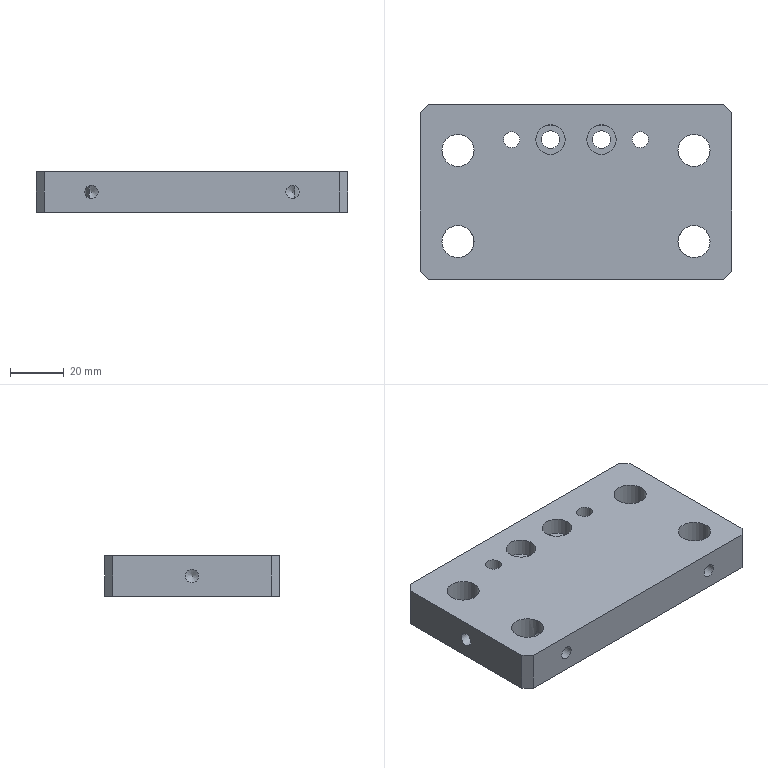Part | NX | features BREP 1 | 1 solid | 29 faces | box 116 x 65 x 15 mm | volume 102539 mm3 | cylinder 14 | plane 12 | cone 3 | commonest cylinder face diameters 5 x4 12 x4 6 x2 6.6 x2 11 x2
STEP:
#1=CARTESIAN_POINT('',(55.,-32.5,0.));
#2=VERTEX_POINT('',#1);
#3=CARTESIAN_POINT('',(58.,-29.5,0.));
#4=VERTEX_POINT('',#3);
#5=CARTESIAN_POINT('',(55.,-32.5,0.));
#6=DIRECTION('',(0.7071,0.7071,0.));
#7=VECTOR('',#6,1000.);
#8=LINE('',#5,#7);
#9=EDGE_CURVE('',#2,#4,#8,.T.);
#10=ORIENTED_EDGE('',*,*,#9,.F.);
#11=CARTESIAN_POINT('',(-55.,-32.5,0.));
#12=VERTEX_POINT('',#11);
#13=CARTESIAN_POINT('',(0.,-32.5,0.));
#14=DIRECTION('',(1.,0.,0.));
#15=VECTOR('',#14,1000.);
#16=LINE('',#13,#15);
#17=EDGE_CURVE('',#12,#2,#16,.T.);
#18=ORIENTED_EDGE('',*,*,#17,.F.);
#19=CARTESIAN_POINT('',(-58.,-29.5,0.));
#20=VERTEX_POINT('',#19);
#21=CARTESIAN_POINT('',(-58.,-29.5,0.));
#22=DIRECTION('',(0.7071,-0.7071,0.));
#23=VECTOR('',#22,1000.);
#24=LINE('',#21,#23);
#25=EDGE_CURVE('',#20,#12,#24,.T.);
#26=ORIENTED_EDGE('',*,*,#25,.F.);
#27=CARTESIAN_POINT('',(-58.,29.5,0.));
#28=VERTEX_POINT('',#27);
#29=CARTESIAN_POINT('',(-58.,0.,0.));
#30=DIRECTION('',(0.,-1.,0.));
#31=VECTOR('',#30,1000.);
#32=LINE('',#29,#31);
#33=EDGE_CURVE('',#28,#20,#32,.T.);
#34=ORIENTED_EDGE('',*,*,#33,.F.);
#35=CARTESIAN_POINT('',(-55.,32.5,0.));
#36=VERTEX_POINT('',#35);
#37=CARTESIAN_POINT('',(-55.,32.5,0.));
#38=DIRECTION('',(-0.7071,-0.7071,0.));
#39=VECTOR('',#38,1000.);
#40=LINE('',#37,#39);
#41=EDGE_CURVE('',#36,#28,#40,.T.);
#42=ORIENTED_EDGE('',*,*,#41,.F.);
#43=CARTESIAN_POINT('',(55.,32.5,0.));
#44=VERTEX_POINT('',#43);
#45=CARTESIAN_POINT('',(0.,32.5,0.));
#46=DIRECTION('',(-1.,0.,0.));
#47=VECTOR('',#46,1000.);
#48=LINE('',#45,#47);
#49=EDGE_CURVE('',#44,#36,#48,.T.);
#50=ORIENTED_EDGE('',*,*,#49,.F.);
#51=CARTESIAN_POINT('',(58.,29.5,0.));
#52=VERTEX_POINT('',#51);
#53=CARTESIAN_POINT('',(58.,29.5,0.));
#54=DIRECTION('',(-0.7071,0.7071,0.));
#55=VECTOR('',#54,1000.);
#56=LINE('',#53,#55);
#57=EDGE_CURVE('',#52,#44,#56,.T.);
#58=ORIENTED_EDGE('',*,*,#57,.F.);
#59=CARTESIAN_POINT('',(58.,0.,0.));
#60=DIRECTION('',(0.,1.,0.));
#61=VECTOR('',#60,1000.);
#62=LINE('',#59,#61);
#63=EDGE_CURVE('',#4,#52,#62,.T.);
#64=ORIENTED_EDGE('',*,*,#63,.F.);
#65=EDGE_LOOP('',(#10,#18,#26,#34,#42,#50,#58,#64));
#66=FACE_BOUND('',#65,.T.);
#67=CARTESIAN_POINT('',(38.,15.5,0.));
#68=VERTEX_POINT('',#67);
#69=CARTESIAN_POINT('',(44.,15.5,0.));
#70=DIRECTION('',(0.,0.,-1.));
#71=DIRECTION('',(-1.,0.,0.));
#72=AXIS2_PLACEMENT_3D('',#69,#70,#71);
#73=CIRCLE('',#72,6.);
#74=EDGE_CURVE('',#68,#68,#73,.T.);
#75=ORIENTED_EDGE('',*,*,#74,.F.);
#76=EDGE_LOOP('',(#75));
#77=FACE_BOUND('',#76,.T.);
#78=CARTESIAN_POINT('',(38.,-18.5,0.));
#79=VERTEX_POINT('',#78);
#80=CARTESIAN_POINT('',(44.,-18.5,0.));
#81=DIRECTION('',(0.,0.,-1.));
#82=DIRECTION('',(-1.,0.,0.));
#83=AXIS2_PLACEMENT_3D('',#80,#81,#82);
#84=CIRCLE('',#83,6.);
#85=EDGE_CURVE('',#79,#79,#84,.T.);
#86=ORIENTED_EDGE('',*,*,#85,.F.);
#87=EDGE_LOOP('',(#86));
#88=FACE_BOUND('',#87,.T.);
#89=CARTESIAN_POINT('',(-50.,-18.5,0.));
#90=VERTEX_POINT('',#89);
#91=CARTESIAN_POINT('',(-44.,-18.5,0.));
#92=DIRECTION('',(0.,0.,-1.));
#93=DIRECTION('',(-1.,0.,0.));
#94=AXIS2_PLACEMENT_3D('',#91,#92,#93);
#95=CIRCLE('',#94,6.);
#96=EDGE_CURVE('',#90,#90,#95,.T.);
#97=ORIENTED_EDGE('',*,*,#96,.F.);
#98=EDGE_LOOP('',(#97));
#99=FACE_BOUND('',#98,.T.);
#100=CARTESIAN_POINT('',(-50.,15.5,0.));
#101=VERTEX_POINT('',#100);
#102=CARTESIAN_POINT('',(-44.,15.5,0.));
#103=DIRECTION('',(0.,0.,-1.));
#104=DIRECTION('',(-1.,0.,0.));
#105=AXIS2_PLACEMENT_3D('',#102,#103,#104);
#106=CIRCLE('',#105,6.);
#107=EDGE_CURVE('',#101,#101,#106,.T.);
#108=ORIENTED_EDGE('',*,*,#107,.F.);
#109=EDGE_LOOP('',(#108));
#110=FACE_BOUND('',#109,.T.);
#111=CARTESIAN_POINT('',(21.,19.5,0.));
#112=VERTEX_POINT('',#111);
#113=CARTESIAN_POINT('',(24.,19.5,0.));
#114=DIRECTION('',(0.,0.,-1.));
#115=DIRECTION('',(-1.,0.,0.));
#116=AXIS2_PLACEMENT_3D('',#113,#114,#115);
#117=CIRCLE('',#116,3.);
#118=EDGE_CURVE('',#112,#112,#117,.T.);
#119=ORIENTED_EDGE('',*,*,#118,.F.);
#120=EDGE_LOOP('',(#119));
#121=FACE_BOUND('',#120,.T.);
#122=CARTESIAN_POINT('',(-27.,19.5,0.));
#123=VERTEX_POINT('',#122);
#124=CARTESIAN_POINT('',(-24.,19.5,0.));
#125=DIRECTION('',(0.,0.,-1.));
#126=DIRECTION('',(-1.,0.,0.));
#127=AXIS2_PLACEMENT_3D('',#124,#125,#126);
#128=CIRCLE('',#127,3.);
#129=EDGE_CURVE('',#123,#123,#128,.T.);
#130=ORIENTED_EDGE('',*,*,#129,.F.);
#131=EDGE_LOOP('',(#130));
#132=FACE_BOUND('',#131,.T.);
#133=CARTESIAN_POINT('',(12.8,19.5,0.));
#134=VERTEX_POINT('',#133);
#135=CARTESIAN_POINT('',(9.5,19.5,0.));
#136=DIRECTION('',(0.,0.,-1.));
#137=DIRECTION('',(1.,0.,0.));
#138=AXIS2_PLACEMENT_3D('',#135,#136,#137);
#139=CIRCLE('',#138,3.3);
#140=EDGE_CURVE('',#134,#134,#139,.T.);
#141=ORIENTED_EDGE('',*,*,#140,.F.);
#142=EDGE_LOOP('',(#141));
#143=FACE_BOUND('',#142,.T.);
#144=CARTESIAN_POINT('',(-6.2,19.5,0.));
#145=VERTEX_POINT('',#144);
#146=CARTESIAN_POINT('',(-9.5,19.5,0.));
#147=DIRECTION('',(0.,0.,-1.));
#148=DIRECTION('',(1.,0.,0.));
#149=AXIS2_PLACEMENT_3D('',#146,#147,#148);
#150=CIRCLE('',#149,3.3);
#151=EDGE_CURVE('',#145,#145,#150,.T.);
#152=ORIENTED_EDGE('',*,*,#151,.F.);
#153=EDGE_LOOP('',(#152));
#154=FACE_BOUND('',#153,.T.);
#155=CARTESIAN_POINT('',(0.,0.,0.));
#156=DIRECTION('',(0.,0.,1.));
#157=DIRECTION('',(-1.,0.,0.));
#158=AXIS2_PLACEMENT_3D('',#155,#156,#157);
#159=PLANE('',#158);
#160=ADVANCED_FACE('',(#66,#77,#88,#99,#110,#121,#132,#143,#154),#159,.F.);
#161=CARTESIAN_POINT('',(58.,-29.5,15.));
#162=VERTEX_POINT('',#161);
#163=CARTESIAN_POINT('',(58.,-29.5,15.));
#164=DIRECTION('',(0.,0.,1.));
#165=VECTOR('',#164,1000.);
#166=LINE('',#163,#165);
#167=EDGE_CURVE('',#4,#162,#166,.T.);
#168=ORIENTED_EDGE('',*,*,#167,.F.);
#169=ORIENTED_EDGE('',*,*,#63,.T.);
#170=CARTESIAN_POINT('',(58.,29.5,15.));
#171=VERTEX_POINT('',#170);
#172=CARTESIAN_POINT('',(58.,29.5,15.));
#173=DIRECTION('',(0.,0.,-1.));
#174=VECTOR('',#173,1000.);
#175=LINE('',#172,#174);
#176=EDGE_CURVE('',#171,#52,#175,.T.);
#177=ORIENTED_EDGE('',*,*,#176,.F.);
#178=CARTESIAN_POINT('',(58.,32.5,15.));
#179=DIRECTION('',(0.,1.,0.));
#180=VECTOR('',#179,1000.);
#181=LINE('',#178,#180);
#182=EDGE_CURVE('',#162,#171,#181,.T.);
#183=ORIENTED_EDGE('',*,*,#182,.F.);
#184=EDGE_LOOP('',(#168,#169,#177,#183));
#185=FACE_BOUND('',#184,.T.);
#186=CARTESIAN_POINT('',(58.,32.5,15.));
#187=DIRECTION('',(-1.,0.,0.));
#188=DIRECTION('',(0.,1.,0.));
#189=AXIS2_PLACEMENT_3D('',#186,#187,#188);
#190=PLANE('',#189);
#191=ADVANCED_FACE('',(#185),#190,.F.);
#192=CARTESIAN_POINT('',(55.,-32.5,15.));
#193=VERTEX_POINT('',#192);
#194=CARTESIAN_POINT('',(55.,-32.5,15.));
#195=DIRECTION('',(0.,0.,1.));
#196=VECTOR('',#195,1000.);
#197=LINE('',#194,#196);
#198=EDGE_CURVE('',#2,#193,#197,.T.);
#199=ORIENTED_EDGE('',*,*,#198,.F.);
#200=ORIENTED_EDGE('',*,*,#9,.T.);
#201=ORIENTED_EDGE('',*,*,#167,.T.);
#202=CARTESIAN_POINT('',(58.,-29.5,15.));
#203=DIRECTION('',(0.7071,0.7071,0.));
#204=VECTOR('',#203,1000.);
#205=LINE('',#202,#204);
#206=EDGE_CURVE('',#193,#162,#205,.T.);
#207=ORIENTED_EDGE('',*,*,#206,.F.);
#208=EDGE_LOOP('',(#199,#200,#201,#207));
#209=FACE_BOUND('',#208,.T.);
#210=CARTESIAN_POINT('',(58.,-29.5,15.));
#211=DIRECTION('',(-0.7071,0.7071,0.));
#212=DIRECTION('',(0.7071,0.7071,0.));
#213=AXIS2_PLACEMENT_3D('',#210,#211,#212);
#214=PLANE('',#213);
#215=ADVANCED_FACE('',(#209),#214,.F.);
#216=ORIENTED_EDGE('',*,*,#198,.T.);
#217=CARTESIAN_POINT('',(-55.,-32.5,15.));
#218=VERTEX_POINT('',#217);
#219=CARTESIAN_POINT('',(-58.,-32.5,15.));
#220=DIRECTION('',(1.,0.,0.));
#221=VECTOR('',#220,1000.);
#222=LINE('',#219,#221);
#223=EDGE_CURVE('',#218,#193,#222,.T.);
#224=ORIENTED_EDGE('',*,*,#223,.F.);
#225=CARTESIAN_POINT('',(-55.,-32.5,15.));
#226=DIRECTION('',(0.,0.,1.));
#227=VECTOR('',#226,1000.);
#228=LINE('',#225,#227);
#229=EDGE_CURVE('',#12,#218,#228,.T.);
#230=ORIENTED_EDGE('',*,*,#229,.F.);
#231=ORIENTED_EDGE('',*,*,#17,.T.);
#232=EDGE_LOOP('',(#216,#224,#230,#231));
#233=FACE_BOUND('',#232,.T.);
#234=CARTESIAN_POINT('',(-37.5,-32.5,5.));
#235=VERTEX_POINT('',#234);
#236=CARTESIAN_POINT('',(-37.5,-32.5,7.5));
#237=DIRECTION('',(0.,-1.,0.));
#238=DIRECTION('',(0.,0.,-1.));
#239=AXIS2_PLACEMENT_3D('',#236,#237,#238);
#240=CIRCLE('',#239,2.5);
#241=EDGE_CURVE('',#235,#235,#240,.T.);
#242=ORIENTED_EDGE('',*,*,#241,.F.);
#243=EDGE_LOOP('',(#242));
#244=FACE_BOUND('',#243,.T.);
#245=CARTESIAN_POINT('',(37.5,-32.5,5.));
#246=VERTEX_POINT('',#245);
#247=CARTESIAN_POINT('',(37.5,-32.5,7.5));
#248=DIRECTION('',(0.,-1.,0.));
#249=DIRECTION('',(0.,0.,-1.));
#250=AXIS2_PLACEMENT_3D('',#247,#248,#249);
#251=CIRCLE('',#250,2.5);
#252=EDGE_CURVE('',#246,#246,#251,.T.);
#253=ORIENTED_EDGE('',*,*,#252,.F.);
#254=EDGE_LOOP('',(#253));
#255=FACE_BOUND('',#254,.T.);
#256=CARTESIAN_POINT('',(-58.,-32.5,15.));
#257=DIRECTION('',(0.,1.,0.));
#258=DIRECTION('',(0.,0.,-1.));
#259=AXIS2_PLACEMENT_3D('',#256,#257,#258);
#260=PLANE('',#259);
#261=ADVANCED_FACE('',(#233,#244,#255),#260,.F.);
#262=CARTESIAN_POINT('',(-58.,-29.5,15.));
#263=VERTEX_POINT('',#262);
#264=CARTESIAN_POINT('',(-58.,-29.5,15.));
#265=DIRECTION('',(0.,0.,1.));
#266=VECTOR('',#265,1000.);
#267=LINE('',#264,#266);
#268=EDGE_CURVE('',#20,#263,#267,.T.);
#269=ORIENTED_EDGE('',*,*,#268,.F.);
#270=ORIENTED_EDGE('',*,*,#25,.T.);
#271=ORIENTED_EDGE('',*,*,#229,.T.);
#272=CARTESIAN_POINT('',(-55.,-32.5,15.));
#273=DIRECTION('',(0.7071,-0.7071,0.));
#274=VECTOR('',#273,1000.);
#275=LINE('',#272,#274);
#276=EDGE_CURVE('',#263,#218,#275,.T.);
#277=ORIENTED_EDGE('',*,*,#276,.F.);
#278=EDGE_LOOP('',(#269,#270,#271,#277));
#279=FACE_BOUND('',#278,.T.);
#280=CARTESIAN_POINT('',(-55.,-32.5,15.));
#281=DIRECTION('',(0.7071,0.7071,0.));
#282=DIRECTION('',(0.7071,-0.7071,0.));
#283=AXIS2_PLACEMENT_3D('',#280,#281,#282);
#284=PLANE('',#283);
#285=ADVANCED_FACE('',(#279),#284,.F.);
#286=CARTESIAN_POINT('',(-58.,29.5,15.));
#287=VERTEX_POINT('',#286);
#288=CARTESIAN_POINT('',(-58.,29.5,15.));
#289=DIRECTION('',(0.,0.,1.));
#290=VECTOR('',#289,1000.);
#291=LINE('',#288,#290);
#292=EDGE_CURVE('',#28,#287,#291,.T.);
#293=ORIENTED_EDGE('',*,*,#292,.F.);
#294=ORIENTED_EDGE('',*,*,#33,.T.);
#295=ORIENTED_EDGE('',*,*,#268,.T.);
#296=CARTESIAN_POINT('',(-58.,32.5,15.));
#297=DIRECTION('',(0.,-1.,0.));
#298=VECTOR('',#297,1000.);
#299=LINE('',#296,#298);
#300=EDGE_CURVE('',#287,#263,#299,.T.);
#301=ORIENTED_EDGE('',*,*,#300,.F.);
#302=EDGE_LOOP('',(#293,#294,#295,#301));
#303=FACE_BOUND('',#302,.T.);
#304=CARTESIAN_POINT('',(-58.,0.,10.));
#305=VERTEX_POINT('',#304);
#306=CARTESIAN_POINT('',(-58.,0.,7.5));
#307=DIRECTION('',(-1.,0.,0.));
#308=DIRECTION('',(0.,0.,1.));
#309=AXIS2_PLACEMENT_3D('',#306,#307,#308);
#310=CIRCLE('',#309,2.5);
#311=EDGE_CURVE('',#305,#305,#310,.T.);
#312=ORIENTED_EDGE('',*,*,#311,.F.);
#313=EDGE_LOOP('',(#312));
#314=FACE_BOUND('',#313,.T.);
#315=CARTESIAN_POINT('',(-58.,32.5,15.));
#316=DIRECTION('',(1.,0.,0.));
#317=DIRECTION('',(0.,-1.,0.));
#318=AXIS2_PLACEMENT_3D('',#315,#316,#317);
#319=PLANE('',#318);
#320=ADVANCED_FACE('',(#303,#314),#319,.F.);
#321=CARTESIAN_POINT('',(-55.,32.5,15.));
#322=VERTEX_POINT('',#321);
#323=CARTESIAN_POINT('',(-55.,32.5,15.));
#324=DIRECTION('',(0.,0.,1.));
#325=VECTOR('',#324,1000.);
#326=LINE('',#323,#325);
#327=EDGE_CURVE('',#36,#322,#326,.T.);
#328=ORIENTED_EDGE('',*,*,#327,.F.);
#329=ORIENTED_EDGE('',*,*,#41,.T.);
#330=ORIENTED_EDGE('',*,*,#292,.T.);
#331=CARTESIAN_POINT('',(-58.,29.5,15.));
#332=DIRECTION('',(-0.7071,-0.7071,0.));
#333=VECTOR('',#332,1000.);
#334=LINE('',#331,#333);
#335=EDGE_CURVE('',#322,#287,#334,.T.);
#336=ORIENTED_EDGE('',*,*,#335,.F.);
#337=EDGE_LOOP('',(#328,#329,#330,#336));
#338=FACE_BOUND('',#337,.T.);
#339=CARTESIAN_POINT('',(-58.,29.5,15.));
#340=DIRECTION('',(0.7071,-0.7071,0.));
#341=DIRECTION('',(-0.7071,-0.7071,0.));
#342=AXIS2_PLACEMENT_3D('',#339,#340,#341);
#343=PLANE('',#342);
#344=ADVANCED_FACE('',(#338),#343,.F.);
#345=CARTESIAN_POINT('',(55.,32.5,15.));
#346=VERTEX_POINT('',#345);
#347=CARTESIAN_POINT('',(55.,32.5,15.));
#348=DIRECTION('',(0.,0.,1.));
#349=VECTOR('',#348,1000.);
#350=LINE('',#347,#349);
#351=EDGE_CURVE('',#44,#346,#350,.T.);
#352=ORIENTED_EDGE('',*,*,#351,.F.);
#353=ORIENTED_EDGE('',*,*,#49,.T.);
#354=ORIENTED_EDGE('',*,*,#327,.T.);
#355=CARTESIAN_POINT('',(-58.,32.5,15.));
#356=DIRECTION('',(-1.,0.,0.));
#357=VECTOR('',#356,1000.);
#358=LINE('',#355,#357);
#359=EDGE_CURVE('',#346,#322,#358,.T.);
#360=ORIENTED_EDGE('',*,*,#359,.F.);
#361=EDGE_LOOP('',(#352,#353,#354,#360));
#362=FACE_BOUND('',#361,.T.);
#363=CARTESIAN_POINT('',(-58.,32.5,15.));
#364=DIRECTION('',(0.,-1.,0.));
#365=DIRECTION('',(0.,0.,1.));
#366=AXIS2_PLACEMENT_3D('',#363,#364,#365);
#367=PLANE('',#366);
#368=ADVANCED_FACE('',(#362),#367,.F.);
#369=ORIENTED_EDGE('',*,*,#176,.T.);
#370=ORIENTED_EDGE('',*,*,#57,.T.);
#371=ORIENTED_EDGE('',*,*,#351,.T.);
#372=CARTESIAN_POINT('',(55.,32.5,15.));
#373=DIRECTION('',(-0.7071,0.7071,0.));
#374=VECTOR('',#373,1000.);
#375=LINE('',#372,#374);
#376=EDGE_CURVE('',#171,#346,#375,.T.);
#377=ORIENTED_EDGE('',*,*,#376,.F.);
#378=EDGE_LOOP('',(#369,#370,#371,#377));
#379=FACE_BOUND('',#378,.T.);
#380=CARTESIAN_POINT('',(55.,32.5,15.));
#381=DIRECTION('',(-0.7071,-0.7071,0.));
#382=DIRECTION('',(-0.7071,0.7071,0.));
#383=AXIS2_PLACEMENT_3D('',#380,#381,#382);
#384=PLANE('',#383);
#385=ADVANCED_FACE('',(#379),#384,.F.);
#386=CARTESIAN_POINT('',(38.,15.5,15.));
#387=VERTEX_POINT('',#386);
#388=CARTESIAN_POINT('',(44.,15.5,15.));
#389=DIRECTION('',(0.,0.,-1.));
#390=DIRECTION('',(-1.,0.,0.));
#391=AXIS2_PLACEMENT_3D('',#388,#389,#390);
#392=CIRCLE('',#391,6.);
#393=EDGE_CURVE('',#387,#387,#392,.T.);
#394=ORIENTED_EDGE('',*,*,#393,.F.);
#395=EDGE_LOOP('',(#394));
#396=FACE_BOUND('',#395,.T.);
#397=ORIENTED_EDGE('',*,*,#74,.T.);
#398=EDGE_LOOP('',(#397));
#399=FACE_BOUND('',#398,.T.);
#400=CARTESIAN_POINT('',(44.,15.5,0.));
#401=DIRECTION('',(0.,0.,-1.));
#402=DIRECTION('',(1.,0.,0.));
#403=AXIS2_PLACEMENT_3D('',#400,#401,#402);
#404=CYLINDRICAL_SURFACE('',#403,6.);
#405=ADVANCED_FACE('',(#396,#399),#404,.F.);
#406=CARTESIAN_POINT('',(38.084,-17.5,5.069));
#407=VERTEX_POINT('',#406);
#408=CARTESIAN_POINT('',(38.084,-17.5,9.931));
#409=VERTEX_POINT('',#408);
#410=CARTESIAN_POINT('',(38.084,-17.5,5.069));
#411=CARTESIAN_POINT('',(38.121,-17.28,5.455));
#412=CARTESIAN_POINT('',(38.219,-16.853,6.213));
#413=CARTESIAN_POINT('',(38.404,-16.329,7.503));
#414=CARTESIAN_POINT('',(38.218,-16.855,8.789));
#415=CARTESIAN_POINT('',(38.121,-17.281,9.546));
#416=CARTESIAN_POINT('',(38.084,-17.5,9.931));
#417=B_SPLINE_CURVE_WITH_KNOTS('',3,(#410,#411,#412,#413,#414,#415,#416),.UNSPECIFIED.,.F.,.F.,(4,1,1,1,4),(0.,0.001335,0.002669,0.004004,0.005339),.UNSPECIFIED.);
#418=EDGE_CURVE('',#407,#409,#417,.T.);
#419=ORIENTED_EDGE('',*,*,#418,.F.);
#420=CARTESIAN_POINT('',(38.084,-17.5,9.931));
#421=CARTESIAN_POINT('',(37.983,-18.098,9.955));
#422=CARTESIAN_POINT('',(37.966,-19.305,9.957));
#423=CARTESIAN_POINT('',(38.461,-21.047,9.846));
#424=CARTESIAN_POINT('',(39.481,-22.542,9.275));
#425=CARTESIAN_POINT('',(40.257,-23.185,7.513));
#426=CARTESIAN_POINT('',(39.492,-22.553,5.735));
#427=CARTESIAN_POINT('',(38.471,-21.068,5.157));
#428=CARTESIAN_POINT('',(37.966,-19.32,5.043));
#429=CARTESIAN_POINT('',(37.983,-18.098,5.045));
#430=CARTESIAN_POINT('',(38.084,-17.5,5.069));
#431=B_SPLINE_CURVE_WITH_KNOTS('',3,(#420,#421,#422,#423,#424,#425,#426,#427,#428,#429,#430),.UNSPECIFIED.,.F.,.F.,(4,1,1,1,1,1,1,1,4),(0.,0.001794,0.003588,0.005381,0.007175,0.008969,0.01076,0.01256,0.01435),.UNSPECIFIED.);
#432=EDGE_CURVE('',#409,#407,#431,.T.);
#433=ORIENTED_EDGE('',*,*,#432,.F.);
#434=EDGE_LOOP('',(#419,#433));
#435=FACE_BOUND('',#434,.T.);
#436=CARTESIAN_POINT('',(38.,-18.5,15.));
#437=VERTEX_POINT('',#436);
#438=CARTESIAN_POINT('',(44.,-18.5,15.));
#439=DIRECTION('',(0.,0.,-1.));
#440=DIRECTION('',(-1.,0.,0.));
#441=AXIS2_PLACEMENT_3D('',#438,#439,#440);
#442=CIRCLE('',#441,6.);
#443=EDGE_CURVE('',#437,#437,#442,.T.);
#444=ORIENTED_EDGE('',*,*,#443,.F.);
#445=EDGE_LOOP('',(#444));
#446=FACE_BOUND('',#445,.T.);
#447=ORIENTED_EDGE('',*,*,#85,.T.);
#448=EDGE_LOOP('',(#447));
#449=FACE_BOUND('',#448,.T.);
#450=CARTESIAN_POINT('',(44.,-18.5,0.));
#451=DIRECTION('',(0.,0.,-1.));
#452=DIRECTION('',(1.,0.,0.));
#453=AXIS2_PLACEMENT_3D('',#450,#451,#452);
#454=CYLINDRICAL_SURFACE('',#453,6.);
#455=ADVANCED_FACE('',(#435,#446,#449),#454,.F.);
#456=ORIENTED_EDGE('',*,*,#96,.T.);
#457=EDGE_LOOP('',(#456));
#458=FACE_BOUND('',#457,.T.);
#459=CARTESIAN_POINT('',(-50.,-18.5,15.));
#460=VERTEX_POINT('',#459);
#461=CARTESIAN_POINT('',(-44.,-18.5,15.));
#462=DIRECTION('',(0.,0.,-1.));
#463=DIRECTION('',(-1.,0.,0.));
#464=AXIS2_PLACEMENT_3D('',#461,#462,#463);
#465=CIRCLE('',#464,6.);
#466=EDGE_CURVE('',#460,#460,#465,.T.);
#467=ORIENTED_EDGE('',*,*,#466,.F.);
#468=EDGE_LOOP('',(#467));
#469=FACE_BOUND('',#468,.T.);
#470=CARTESIAN_POINT('',(-38.084,-17.5,9.931));
#471=VERTEX_POINT('',#470);
#472=CARTESIAN_POINT('',(-38.084,-17.5,5.069));
#473=VERTEX_POINT('',#472);
#474=CARTESIAN_POINT('',(-38.084,-17.5,9.931));
#475=CARTESIAN_POINT('',(-38.121,-17.28,9.545));
#476=CARTESIAN_POINT('',(-38.219,-16.853,8.787));
#477=CARTESIAN_POINT('',(-38.404,-16.329,7.497));
#478=CARTESIAN_POINT('',(-38.218,-16.855,6.211));
#479=CARTESIAN_POINT('',(-38.121,-17.281,5.454));
#480=CARTESIAN_POINT('',(-38.084,-17.5,5.069));
#481=B_SPLINE_CURVE_WITH_KNOTS('',3,(#474,#475,#476,#477,#478,#479,#480),.UNSPECIFIED.,.F.,.F.,(4,1,1,1,4),(0.,0.001335,0.002669,0.004004,0.005339),.UNSPECIFIED.);
#482=EDGE_CURVE('',#471,#473,#481,.T.);
#483=ORIENTED_EDGE('',*,*,#482,.F.);
#484=CARTESIAN_POINT('',(-38.084,-17.5,5.069));
#485=CARTESIAN_POINT('',(-37.983,-18.098,5.045));
#486=CARTESIAN_POINT('',(-37.966,-19.305,5.043));
#487=CARTESIAN_POINT('',(-38.461,-21.047,5.154));
#488=CARTESIAN_POINT('',(-39.481,-22.542,5.725));
#489=CARTESIAN_POINT('',(-40.257,-23.185,7.487));
#490=CARTESIAN_POINT('',(-39.492,-22.553,9.265));
#491=CARTESIAN_POINT('',(-38.471,-21.068,9.843));
#492=CARTESIAN_POINT('',(-37.966,-19.32,9.957));
#493=CARTESIAN_POINT('',(-37.983,-18.098,9.955));
#494=CARTESIAN_POINT('',(-38.084,-17.5,9.931));
#495=B_SPLINE_CURVE_WITH_KNOTS('',3,(#484,#485,#486,#487,#488,#489,#490,#491,#492,#493,#494),.UNSPECIFIED.,.F.,.F.,(4,1,1,1,1,1,1,1,4),(0.,0.001794,0.003588,0.005381,0.007175,0.008969,0.01076,0.01256,0.01435),.UNSPECIFIED.);
#496=EDGE_CURVE('',#473,#471,#495,.T.);
#497=ORIENTED_EDGE('',*,*,#496,.F.);
#498=EDGE_LOOP('',(#483,#497));
#499=FACE_BOUND('',#498,.T.);
#500=CARTESIAN_POINT('',(-44.,-18.5,0.));
#501=DIRECTION('',(0.,0.,-1.));
#502=DIRECTION('',(1.,0.,0.));
#503=AXIS2_PLACEMENT_3D('',#500,#501,#502);
#504=CYLINDRICAL_SURFACE('',#503,6.);
#505=ADVANCED_FACE('',(#458,#469,#499),#504,.F.);
#506=CARTESIAN_POINT('',(-50.,15.5,15.));
#507=VERTEX_POINT('',#506);
#508=CARTESIAN_POINT('',(-44.,15.5,15.));
#509=DIRECTION('',(0.,0.,-1.));
#510=DIRECTION('',(-1.,0.,0.));
#511=AXIS2_PLACEMENT_3D('',#508,#509,#510);
#512=CIRCLE('',#511,6.);
#513=EDGE_CURVE('',#507,#507,#512,.T.);
#514=ORIENTED_EDGE('',*,*,#513,.F.);
#515=EDGE_LOOP('',(#514));
#516=FACE_BOUND('',#515,.T.);
#517=ORIENTED_EDGE('',*,*,#107,.T.);
#518=EDGE_LOOP('',(#517));
#519=FACE_BOUND('',#518,.T.);
#520=CARTESIAN_POINT('',(-44.,15.5,0.));
#521=DIRECTION('',(0.,0.,-1.));
#522=DIRECTION('',(1.,0.,0.));
#523=AXIS2_PLACEMENT_3D('',#520,#521,#522);
#524=CYLINDRICAL_SURFACE('',#523,6.);
#525=ADVANCED_FACE('',(#516,#519),#524,.F.);
#526=CARTESIAN_POINT('',(21.,19.5,15.));
#527=VERTEX_POINT('',#526);
#528=CARTESIAN_POINT('',(24.,19.5,15.));
#529=DIRECTION('',(0.,0.,-1.));
#530=DIRECTION('',(-1.,0.,0.));
#531=AXIS2_PLACEMENT_3D('',#528,#529,#530);
#532=CIRCLE('',#531,3.);
#533=EDGE_CURVE('',#527,#527,#532,.T.);
#534=ORIENTED_EDGE('',*,*,#533,.F.);
#535=EDGE_LOOP('',(#534));
#536=FACE_BOUND('',#535,.T.);
#537=ORIENTED_EDGE('',*,*,#118,.T.);
#538=EDGE_LOOP('',(#537));
#539=FACE_BOUND('',#538,.T.);
#540=CARTESIAN_POINT('',(24.,19.5,0.));
#541=DIRECTION('',(0.,0.,-1.));
#542=DIRECTION('',(1.,0.,0.));
#543=AXIS2_PLACEMENT_3D('',#540,#541,#542);
#544=CYLINDRICAL_SURFACE('',#543,3.);
#545=ADVANCED_FACE('',(#536,#539),#544,.F.);
#546=CARTESIAN_POINT('',(-27.,19.5,15.));
#547=VERTEX_POINT('',#546);
#548=CARTESIAN_POINT('',(-24.,19.5,15.));
#549=DIRECTION('',(0.,0.,-1.));
#550=DIRECTION('',(-1.,0.,0.));
#551=AXIS2_PLACEMENT_3D('',#548,#549,#550);
#552=CIRCLE('',#551,3.);
#553=EDGE_CURVE('',#547,#547,#552,.T.);
#554=ORIENTED_EDGE('',*,*,#553,.F.);
#555=EDGE_LOOP('',(#554));
#556=FACE_BOUND('',#555,.T.);
#557=ORIENTED_EDGE('',*,*,#129,.T.);
#558=EDGE_LOOP('',(#557));
#559=FACE_BOUND('',#558,.T.);
#560=CARTESIAN_POINT('',(-24.,19.5,0.));
#561=DIRECTION('',(0.,0.,-1.));
#562=DIRECTION('',(1.,0.,0.));
#563=AXIS2_PLACEMENT_3D('',#560,#561,#562);
#564=CYLINDRICAL_SURFACE('',#563,3.);
#565=ADVANCED_FACE('',(#556,#559),#564,.F.);
#566=ORIENTED_EDGE('',*,*,#140,.T.);
#567=EDGE_LOOP('',(#566));
#568=FACE_BOUND('',#567,.T.);
#569=CARTESIAN_POINT('',(12.8,19.5,8.6));
#570=VERTEX_POINT('',#569);
#571=CARTESIAN_POINT('',(9.5,19.5,8.6));
#572=DIRECTION('',(0.,0.,-1.));
#573=DIRECTION('',(1.,0.,0.));
#574=AXIS2_PLACEMENT_3D('',#571,#572,#573);
#575=CIRCLE('',#574,3.3);
#576=EDGE_CURVE('',#570,#570,#575,.T.);
#577=ORIENTED_EDGE('',*,*,#576,.F.);
#578=EDGE_LOOP('',(#577));
#579=FACE_BOUND('',#578,.T.);
#580=CARTESIAN_POINT('',(9.5,19.5,15.));
#581=DIRECTION('',(0.,0.,1.));
#582=DIRECTION('',(-1.,0.,0.));
#583=AXIS2_PLACEMENT_3D('',#580,#581,#582);
#584=CYLINDRICAL_SURFACE('',#583,3.3);
#585=ADVANCED_FACE('',(#568,#579),#584,.F.);
#586=ORIENTED_EDGE('',*,*,#151,.T.);
#587=EDGE_LOOP('',(#586));
#588=FACE_BOUND('',#587,.T.);
#589=CARTESIAN_POINT('',(-6.2,19.5,8.6));
#590=VERTEX_POINT('',#589);
#591=CARTESIAN_POINT('',(-9.5,19.5,8.6));
#592=DIRECTION('',(0.,0.,-1.));
#593=DIRECTION('',(1.,0.,0.));
#594=AXIS2_PLACEMENT_3D('',#591,#592,#593);
#595=CIRCLE('',#594,3.3);
#596=EDGE_CURVE('',#590,#590,#595,.T.);
#597=ORIENTED_EDGE('',*,*,#596,.F.);
#598=EDGE_LOOP('',(#597));
#599=FACE_BOUND('',#598,.T.);
#600=CARTESIAN_POINT('',(-9.5,19.5,15.));
#601=DIRECTION('',(0.,0.,1.));
#602=DIRECTION('',(-1.,0.,0.));
#603=AXIS2_PLACEMENT_3D('',#600,#601,#602);
#604=CYLINDRICAL_SURFACE('',#603,3.3);
#605=ADVANCED_FACE('',(#588,#599),#604,.F.);
#606=ORIENTED_EDGE('',*,*,#300,.T.);
#607=ORIENTED_EDGE('',*,*,#276,.T.);
#608=ORIENTED_EDGE('',*,*,#223,.T.);
#609=ORIENTED_EDGE('',*,*,#206,.T.);
#610=ORIENTED_EDGE('',*,*,#182,.T.);
#611=ORIENTED_EDGE('',*,*,#376,.T.);
#612=ORIENTED_EDGE('',*,*,#359,.T.);
#613=ORIENTED_EDGE('',*,*,#335,.T.);
#614=EDGE_LOOP('',(#606,#607,#608,#609,#610,#611,#612,#613));
#615=FACE_BOUND('',#614,.T.);
#616=ORIENTED_EDGE('',*,*,#393,.T.);
#617=EDGE_LOOP('',(#616));
#618=FACE_BOUND('',#617,.T.);
#619=ORIENTED_EDGE('',*,*,#443,.T.);
#620=EDGE_LOOP('',(#619));
#621=FACE_BOUND('',#620,.T.);
#622=ORIENTED_EDGE('',*,*,#466,.T.);
#623=EDGE_LOOP('',(#622));
#624=FACE_BOUND('',#623,.T.);
#625=ORIENTED_EDGE('',*,*,#513,.T.);
#626=EDGE_LOOP('',(#625));
#627=FACE_BOUND('',#626,.T.);
#628=ORIENTED_EDGE('',*,*,#533,.T.);
#629=EDGE_LOOP('',(#628));
#630=FACE_BOUND('',#629,.T.);
#631=ORIENTED_EDGE('',*,*,#553,.T.);
#632=EDGE_LOOP('',(#631));
#633=FACE_BOUND('',#632,.T.);
#634=CARTESIAN_POINT('',(15.,19.5,15.));
#635=VERTEX_POINT('',#634);
#636=CARTESIAN_POINT('',(9.5,19.5,15.));
#637=DIRECTION('',(0.,0.,-1.));
#638=DIRECTION('',(1.,0.,0.));
#639=AXIS2_PLACEMENT_3D('',#636,#637,#638);
#640=CIRCLE('',#639,5.5);
#641=EDGE_CURVE('',#635,#635,#640,.T.);
#642=ORIENTED_EDGE('',*,*,#641,.T.);
#643=EDGE_LOOP('',(#642));
#644=FACE_BOUND('',#643,.T.);
#645=CARTESIAN_POINT('',(-4.,19.5,15.));
#646=VERTEX_POINT('',#645);
#647=CARTESIAN_POINT('',(-9.5,19.5,15.));
#648=DIRECTION('',(0.,0.,-1.));
#649=DIRECTION('',(1.,0.,0.));
#650=AXIS2_PLACEMENT_3D('',#647,#648,#649);
#651=CIRCLE('',#650,5.5);
#652=EDGE_CURVE('',#646,#646,#651,.T.);
#653=ORIENTED_EDGE('',*,*,#652,.T.);
#654=EDGE_LOOP('',(#653));
#655=FACE_BOUND('',#654,.T.);
#656=CARTESIAN_POINT('',(0.,0.,15.));
#657=DIRECTION('',(0.,0.,1.));
#658=DIRECTION('',(-1.,0.,0.));
#659=AXIS2_PLACEMENT_3D('',#656,#657,#658);
#660=PLANE('',#659);
#661=ADVANCED_FACE('',(#615,#618,#621,#624,#627,#630,#633,#644,#655),#660,.T.);
#662=CARTESIAN_POINT('',(-37.5,-17.5,7.5));
#663=DIRECTION('',(0.,-1.,0.));
#664=DIRECTION('',(0.,0.,-1.));
#665=AXIS2_PLACEMENT_3D('',#662,#663,#664);
#666=CIRCLE('',#665,2.5);
#667=EDGE_CURVE('',#473,#471,#666,.T.);
#668=ORIENTED_EDGE('',*,*,#667,.F.);
#669=ORIENTED_EDGE('',*,*,#496,.T.);
#670=EDGE_LOOP('',(#668,#669));
#671=FACE_BOUND('',#670,.T.);
#672=ORIENTED_EDGE('',*,*,#241,.T.);
#673=EDGE_LOOP('',(#672));
#674=FACE_BOUND('',#673,.T.);
#675=CARTESIAN_POINT('',(-37.5,-32.5,7.5));
#676=DIRECTION('',(0.,-1.,0.));
#677=DIRECTION('',(0.,0.,1.));
#678=AXIS2_PLACEMENT_3D('',#675,#676,#677);
#679=CYLINDRICAL_SURFACE('',#678,2.5);
#680=ADVANCED_FACE('',(#671,#674),#679,.F.);
#681=ORIENTED_EDGE('',*,*,#432,.T.);
#682=CARTESIAN_POINT('',(37.5,-17.5,7.5));
#683=DIRECTION('',(0.,-1.,0.));
#684=DIRECTION('',(0.,0.,-1.));
#685=AXIS2_PLACEMENT_3D('',#682,#683,#684);
#686=CIRCLE('',#685,2.5);
#687=EDGE_CURVE('',#409,#407,#686,.T.);
#688=ORIENTED_EDGE('',*,*,#687,.F.);
#689=EDGE_LOOP('',(#681,#688));
#690=FACE_BOUND('',#689,.T.);
#691=ORIENTED_EDGE('',*,*,#252,.T.);
#692=EDGE_LOOP('',(#691));
#693=FACE_BOUND('',#692,.T.);
#694=CARTESIAN_POINT('',(37.5,-32.5,7.5));
#695=DIRECTION('',(0.,-1.,0.));
#696=DIRECTION('',(0.,0.,1.));
#697=AXIS2_PLACEMENT_3D('',#694,#695,#696);
#698=CYLINDRICAL_SURFACE('',#697,2.5);
#699=ADVANCED_FACE('',(#690,#693),#698,.F.);
#700=CARTESIAN_POINT('',(-43.,0.,10.));
#701=VERTEX_POINT('',#700);
#702=CARTESIAN_POINT('',(-43.,0.,7.5));
#703=DIRECTION('',(-1.,0.,0.));
#704=DIRECTION('',(0.,0.,1.));
#705=AXIS2_PLACEMENT_3D('',#702,#703,#704);
#706=CIRCLE('',#705,2.5);
#707=EDGE_CURVE('',#701,#701,#706,.T.);
#708=ORIENTED_EDGE('',*,*,#707,.F.);
#709=EDGE_LOOP('',(#708));
#710=FACE_BOUND('',#709,.T.);
#711=ORIENTED_EDGE('',*,*,#311,.T.);
#712=EDGE_LOOP('',(#711));
#713=FACE_BOUND('',#712,.T.);
#714=CARTESIAN_POINT('',(-58.,0.,7.5));
#715=DIRECTION('',(-1.,0.,0.));
#716=DIRECTION('',(0.,0.,-1.));
#717=AXIS2_PLACEMENT_3D('',#714,#715,#716);
#718=CYLINDRICAL_SURFACE('',#717,2.5);
#719=ADVANCED_FACE('',(#710,#713),#718,.F.);
#720=ORIENTED_EDGE('',*,*,#687,.T.);
#721=ORIENTED_EDGE('',*,*,#418,.T.);
#722=EDGE_LOOP('',(#720,#721));
#723=FACE_BOUND('',#722,.T.);
#724=CARTESIAN_POINT('',(37.5,-17.5,7.5));
#725=DIRECTION('',(0.,-1.,0.));
#726=DIRECTION('',(0.,0.,1.));
#727=AXIS2_PLACEMENT_3D('',#724,#725,#726);
#728=CONICAL_SURFACE('',#727,2.5,1.03);
#729=ADVANCED_FACE('',(#723),#728,.F.);
#730=ORIENTED_EDGE('',*,*,#667,.T.);
#731=ORIENTED_EDGE('',*,*,#482,.T.);
#732=EDGE_LOOP('',(#730,#731));
#733=FACE_BOUND('',#732,.T.);
#734=CARTESIAN_POINT('',(-37.5,-17.5,7.5));
#735=DIRECTION('',(0.,-1.,0.));
#736=DIRECTION('',(0.,0.,1.));
#737=AXIS2_PLACEMENT_3D('',#734,#735,#736);
#738=CONICAL_SURFACE('',#737,2.5,1.03);
#739=ADVANCED_FACE('',(#733),#738,.F.);
#740=CARTESIAN_POINT('',(15.,19.5,8.6));
#741=VERTEX_POINT('',#740);
#742=CARTESIAN_POINT('',(9.5,19.5,8.6));
#743=DIRECTION('',(0.,0.,-1.));
#744=DIRECTION('',(1.,0.,0.));
#745=AXIS2_PLACEMENT_3D('',#742,#743,#744);
#746=CIRCLE('',#745,5.5);
#747=EDGE_CURVE('',#741,#741,#746,.T.);
#748=ORIENTED_EDGE('',*,*,#747,.F.);
#749=EDGE_LOOP('',(#748));
#750=FACE_BOUND('',#749,.T.);
#751=ORIENTED_EDGE('',*,*,#576,.T.);
#752=EDGE_LOOP('',(#751));
#753=FACE_BOUND('',#752,.T.);
#754=CARTESIAN_POINT('',(12.8,19.5,8.6));
#755=DIRECTION('',(0.,0.,-1.));
#756=DIRECTION('',(1.,0.,0.));
#757=AXIS2_PLACEMENT_3D('',#754,#755,#756);
#758=PLANE('',#757);
#759=ADVANCED_FACE('',(#750,#753),#758,.F.);
#760=CARTESIAN_POINT('',(-4.,19.5,8.6));
#761=VERTEX_POINT('',#760);
#762=CARTESIAN_POINT('',(-9.5,19.5,8.6));
#763=DIRECTION('',(0.,0.,-1.));
#764=DIRECTION('',(1.,0.,0.));
#765=AXIS2_PLACEMENT_3D('',#762,#763,#764);
#766=CIRCLE('',#765,5.5);
#767=EDGE_CURVE('',#761,#761,#766,.T.);
#768=ORIENTED_EDGE('',*,*,#767,.F.);
#769=EDGE_LOOP('',(#768));
#770=FACE_BOUND('',#769,.T.);
#771=ORIENTED_EDGE('',*,*,#596,.T.);
#772=EDGE_LOOP('',(#771));
#773=FACE_BOUND('',#772,.T.);
#774=CARTESIAN_POINT('',(-6.2,19.5,8.6));
#775=DIRECTION('',(0.,0.,-1.));
#776=DIRECTION('',(1.,0.,0.));
#777=AXIS2_PLACEMENT_3D('',#774,#775,#776);
#778=PLANE('',#777);
#779=ADVANCED_FACE('',(#770,#773),#778,.F.);
#780=ORIENTED_EDGE('',*,*,#641,.F.);
#781=EDGE_LOOP('',(#780));
#782=FACE_BOUND('',#781,.T.);
#783=ORIENTED_EDGE('',*,*,#747,.T.);
#784=EDGE_LOOP('',(#783));
#785=FACE_BOUND('',#784,.T.);
#786=CARTESIAN_POINT('',(9.5,19.5,15.));
#787=DIRECTION('',(0.,0.,1.));
#788=DIRECTION('',(-1.,0.,0.));
#789=AXIS2_PLACEMENT_3D('',#786,#787,#788);
#790=CYLINDRICAL_SURFACE('',#789,5.5);
#791=ADVANCED_FACE('',(#782,#785),#790,.F.);
#792=ORIENTED_EDGE('',*,*,#652,.F.);
#793=EDGE_LOOP('',(#792));
#794=FACE_BOUND('',#793,.T.);
#795=ORIENTED_EDGE('',*,*,#767,.T.);
#796=EDGE_LOOP('',(#795));
#797=FACE_BOUND('',#796,.T.);
#798=CARTESIAN_POINT('',(-9.5,19.5,15.));
#799=DIRECTION('',(0.,0.,1.));
#800=DIRECTION('',(-1.,0.,0.));
#801=AXIS2_PLACEMENT_3D('',#798,#799,#800);
#802=CYLINDRICAL_SURFACE('',#801,5.5);
#803=ADVANCED_FACE('',(#794,#797),#802,.F.);
#804=CARTESIAN_POINT('',(-41.498,0.,7.5));
#805=VERTEX_POINT('',#804);
#806=VERTEX_LOOP('',#805);
#807=FACE_BOUND('',#806,.T.);
#808=ORIENTED_EDGE('',*,*,#707,.T.);
#809=EDGE_LOOP('',(#808));
#810=FACE_BOUND('',#809,.T.);
#811=CARTESIAN_POINT('',(-43.,0.,7.5));
#812=DIRECTION('',(-1.,0.,0.));
#813=DIRECTION('',(0.,0.,-1.));
#814=AXIS2_PLACEMENT_3D('',#811,#812,#813);
#815=CONICAL_SURFACE('',#814,2.5,1.03);
#816=ADVANCED_FACE('',(#807,#810),#815,.F.);
#817=CLOSED_SHELL('',(#160,#191,#215,#261,#285,#320,#344,#368,#385,#405,#455,#505,#525,#545,#565,#585,#605,#661,#680,#699,#719,#729,#739,#759,#779,#791,#803,#816));
#818=MANIFOLD_SOLID_BREP('',#817);
#819=(LENGTH_UNIT()NAMED_UNIT(*)SI_UNIT(.MILLI.,.METRE.));
#820=UNCERTAINTY_MEASURE_WITH_UNIT(LENGTH_MEASURE(0.0508),#819,'','');
#821=(NAMED_UNIT(*)PLANE_ANGLE_UNIT()SI_UNIT($,.RADIAN.));
#822=(NAMED_UNIT(*)SI_UNIT($,.STERADIAN.)SOLID_ANGLE_UNIT());
#823=(GEOMETRIC_REPRESENTATION_CONTEXT(3)GLOBAL_UNCERTAINTY_ASSIGNED_CONTEXT((#820))GLOBAL_UNIT_ASSIGNED_CONTEXT((#819,#821,#822))REPRESENTATION_CONTEXT('',''));
#824=ADVANCED_BREP_SHAPE_REPRESENTATION('',(#818),#823);